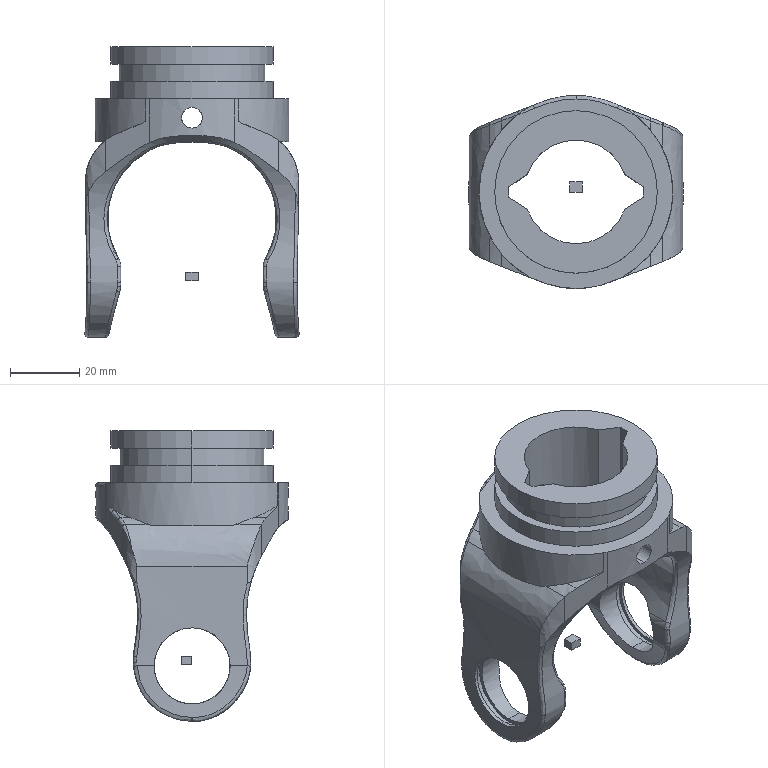Part | STEP file | CARDAN_1PARTV11 | 2 solids | 196 faces | box 61.98 x 55.8 x 84.032 mm | volume 60025 mm3 | spline 127 | cylinder 36 | plane 28 | sphere 4 | torus 1 | commonest cylinder face diameters 2 x9 22 x8 6 x4 24 x4 47 x4 56 x3